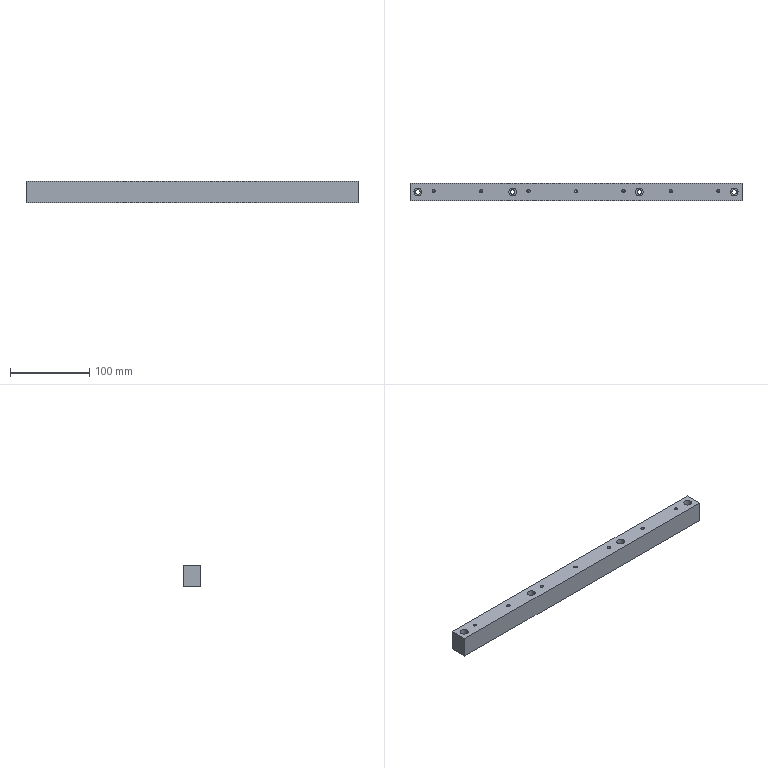Part | SolidWorks | features HoleWzd 2, Extrusion 1 | 1 solid | 54 faces | box 420 x 22 x 27 mm | volume 241946 mm3 | cylinder 30 | cone 14 | plane 10 | commonest cylinder face diameters 4.2 x14 5.5 x8 10 x8
STEP:
#1=CARTESIAN_POINT('',(-205.,0.,10.));
#2=VERTEX_POINT('',#1);
#3=CARTESIAN_POINT('',(-195.,0.,10.));
#4=VERTEX_POINT('',#3);
#5=CARTESIAN_POINT('',(-200.,0.,10.));
#6=DIRECTION('',(0.,0.,1.));
#7=DIRECTION('',(1.,0.,0.));
#8=AXIS2_PLACEMENT_3D('',#5,#6,#7);
#9=CIRCLE('',#8,5.);
#10=EDGE_CURVE('',#2,#4,#9,.T.);
#11=ORIENTED_EDGE('',*,*,#10,.F.);
#12=CARTESIAN_POINT('',(-205.,0.,27.));
#13=VERTEX_POINT('',#12);
#14=CARTESIAN_POINT('',(-205.,0.,27.));
#15=DIRECTION('',(0.,0.,1.));
#16=VECTOR('',#15,1000.);
#17=LINE('',#14,#16);
#18=EDGE_CURVE('',#2,#13,#17,.T.);
#19=ORIENTED_EDGE('',*,*,#18,.T.);
#20=CARTESIAN_POINT('',(-195.,0.,27.));
#21=VERTEX_POINT('',#20);
#22=CARTESIAN_POINT('',(-200.,0.,27.));
#23=DIRECTION('',(0.,0.,1.));
#24=DIRECTION('',(1.,0.,0.));
#25=AXIS2_PLACEMENT_3D('',#22,#23,#24);
#26=CIRCLE('',#25,5.);
#27=EDGE_CURVE('',#13,#21,#26,.T.);
#28=ORIENTED_EDGE('',*,*,#27,.T.);
#29=CARTESIAN_POINT('',(-195.,0.,27.));
#30=DIRECTION('',(0.,0.,1.));
#31=VECTOR('',#30,1000.);
#32=LINE('',#29,#31);
#33=EDGE_CURVE('',#4,#21,#32,.T.);
#34=ORIENTED_EDGE('',*,*,#33,.F.);
#35=EDGE_LOOP('',(#11,#19,#28,#34));
#36=FACE_OUTER_BOUND('',#35,.T.);
#37=CARTESIAN_POINT('',(-200.,0.,27.));
#38=DIRECTION('',(0.,0.,1.));
#39=DIRECTION('',(1.,0.,0.));
#40=AXIS2_PLACEMENT_3D('',#37,#38,#39);
#41=CYLINDRICAL_SURFACE('',#40,5.);
#42=ADVANCED_FACE('',(#36),#41,.F.);
#43=CARTESIAN_POINT('',(-202.75,0.,0.));
#44=VERTEX_POINT('',#43);
#45=CARTESIAN_POINT('',(-197.25,0.,0.));
#46=VERTEX_POINT('',#45);
#47=CARTESIAN_POINT('',(-200.,0.,0.));
#48=DIRECTION('',(0.,0.,1.));
#49=DIRECTION('',(1.,0.,0.));
#50=AXIS2_PLACEMENT_3D('',#47,#48,#49);
#51=CIRCLE('',#50,2.75);
#52=EDGE_CURVE('',#44,#46,#51,.T.);
#53=ORIENTED_EDGE('',*,*,#52,.F.);
#54=CARTESIAN_POINT('',(-202.75,0.,10.));
#55=VERTEX_POINT('',#54);
#56=CARTESIAN_POINT('',(-202.75,0.,27.));
#57=DIRECTION('',(0.,0.,1.));
#58=VECTOR('',#57,1000.);
#59=LINE('',#56,#58);
#60=EDGE_CURVE('',#44,#55,#59,.T.);
#61=ORIENTED_EDGE('',*,*,#60,.T.);
#62=CARTESIAN_POINT('',(-197.25,0.,10.));
#63=VERTEX_POINT('',#62);
#64=CARTESIAN_POINT('',(-200.,0.,10.));
#65=DIRECTION('',(0.,0.,1.));
#66=DIRECTION('',(1.,0.,0.));
#67=AXIS2_PLACEMENT_3D('',#64,#65,#66);
#68=CIRCLE('',#67,2.75);
#69=EDGE_CURVE('',#55,#63,#68,.T.);
#70=ORIENTED_EDGE('',*,*,#69,.T.);
#71=CARTESIAN_POINT('',(-197.25,0.,27.));
#72=DIRECTION('',(0.,0.,1.));
#73=VECTOR('',#72,1000.);
#74=LINE('',#71,#73);
#75=EDGE_CURVE('',#46,#63,#74,.T.);
#76=ORIENTED_EDGE('',*,*,#75,.F.);
#77=EDGE_LOOP('',(#53,#61,#70,#76));
#78=FACE_OUTER_BOUND('',#77,.T.);
#79=CARTESIAN_POINT('',(-200.,0.,27.));
#80=DIRECTION('',(0.,0.,1.));
#81=DIRECTION('',(1.,0.,0.));
#82=AXIS2_PLACEMENT_3D('',#79,#80,#81);
#83=CYLINDRICAL_SURFACE('',#82,2.75);
#84=ADVANCED_FACE('',(#78),#83,.F.);
#85=CARTESIAN_POINT('',(-85.,0.,10.));
#86=VERTEX_POINT('',#85);
#87=CARTESIAN_POINT('',(-75.,0.,10.));
#88=VERTEX_POINT('',#87);
#89=CARTESIAN_POINT('',(-80.,0.,10.));
#90=DIRECTION('',(0.,0.,1.));
#91=DIRECTION('',(1.,0.,0.));
#92=AXIS2_PLACEMENT_3D('',#89,#90,#91);
#93=CIRCLE('',#92,5.);
#94=EDGE_CURVE('',#86,#88,#93,.T.);
#95=ORIENTED_EDGE('',*,*,#94,.F.);
#96=CARTESIAN_POINT('',(-85.,0.,27.));
#97=VERTEX_POINT('',#96);
#98=CARTESIAN_POINT('',(-85.,0.,27.));
#99=DIRECTION('',(0.,0.,1.));
#100=VECTOR('',#99,1000.);
#101=LINE('',#98,#100);
#102=EDGE_CURVE('',#86,#97,#101,.T.);
#103=ORIENTED_EDGE('',*,*,#102,.T.);
#104=CARTESIAN_POINT('',(-75.,0.,27.));
#105=VERTEX_POINT('',#104);
#106=CARTESIAN_POINT('',(-80.,0.,27.));
#107=DIRECTION('',(0.,0.,1.));
#108=DIRECTION('',(1.,0.,0.));
#109=AXIS2_PLACEMENT_3D('',#106,#107,#108);
#110=CIRCLE('',#109,5.);
#111=EDGE_CURVE('',#97,#105,#110,.T.);
#112=ORIENTED_EDGE('',*,*,#111,.T.);
#113=CARTESIAN_POINT('',(-75.,0.,27.));
#114=DIRECTION('',(0.,0.,1.));
#115=VECTOR('',#114,1000.);
#116=LINE('',#113,#115);
#117=EDGE_CURVE('',#88,#105,#116,.T.);
#118=ORIENTED_EDGE('',*,*,#117,.F.);
#119=EDGE_LOOP('',(#95,#103,#112,#118));
#120=FACE_OUTER_BOUND('',#119,.T.);
#121=CARTESIAN_POINT('',(-80.,0.,27.));
#122=DIRECTION('',(0.,0.,1.));
#123=DIRECTION('',(1.,0.,0.));
#124=AXIS2_PLACEMENT_3D('',#121,#122,#123);
#125=CYLINDRICAL_SURFACE('',#124,5.);
#126=ADVANCED_FACE('',(#120),#125,.F.);
#127=CARTESIAN_POINT('',(-82.75,0.,0.));
#128=VERTEX_POINT('',#127);
#129=CARTESIAN_POINT('',(-77.25,0.,0.));
#130=VERTEX_POINT('',#129);
#131=CARTESIAN_POINT('',(-80.,0.,0.));
#132=DIRECTION('',(0.,0.,1.));
#133=DIRECTION('',(1.,0.,0.));
#134=AXIS2_PLACEMENT_3D('',#131,#132,#133);
#135=CIRCLE('',#134,2.75);
#136=EDGE_CURVE('',#128,#130,#135,.T.);
#137=ORIENTED_EDGE('',*,*,#136,.F.);
#138=CARTESIAN_POINT('',(-82.75,0.,10.));
#139=VERTEX_POINT('',#138);
#140=CARTESIAN_POINT('',(-82.75,0.,27.));
#141=DIRECTION('',(0.,0.,1.));
#142=VECTOR('',#141,1000.);
#143=LINE('',#140,#142);
#144=EDGE_CURVE('',#128,#139,#143,.T.);
#145=ORIENTED_EDGE('',*,*,#144,.T.);
#146=CARTESIAN_POINT('',(-77.25,0.,10.));
#147=VERTEX_POINT('',#146);
#148=CARTESIAN_POINT('',(-80.,0.,10.));
#149=DIRECTION('',(0.,0.,1.));
#150=DIRECTION('',(1.,0.,0.));
#151=AXIS2_PLACEMENT_3D('',#148,#149,#150);
#152=CIRCLE('',#151,2.75);
#153=EDGE_CURVE('',#139,#147,#152,.T.);
#154=ORIENTED_EDGE('',*,*,#153,.T.);
#155=CARTESIAN_POINT('',(-77.25,0.,27.));
#156=DIRECTION('',(0.,0.,1.));
#157=VECTOR('',#156,1000.);
#158=LINE('',#155,#157);
#159=EDGE_CURVE('',#130,#147,#158,.T.);
#160=ORIENTED_EDGE('',*,*,#159,.F.);
#161=EDGE_LOOP('',(#137,#145,#154,#160));
#162=FACE_OUTER_BOUND('',#161,.T.);
#163=CARTESIAN_POINT('',(-80.,0.,27.));
#164=DIRECTION('',(0.,0.,1.));
#165=DIRECTION('',(1.,0.,0.));
#166=AXIS2_PLACEMENT_3D('',#163,#164,#165);
#167=CYLINDRICAL_SURFACE('',#166,2.75);
#168=ADVANCED_FACE('',(#162),#167,.F.);
#169=CARTESIAN_POINT('',(75.,0.,10.));
#170=VERTEX_POINT('',#169);
#171=CARTESIAN_POINT('',(85.,0.,10.));
#172=VERTEX_POINT('',#171);
#173=CARTESIAN_POINT('',(80.,0.,10.));
#174=DIRECTION('',(0.,0.,1.));
#175=DIRECTION('',(1.,0.,0.));
#176=AXIS2_PLACEMENT_3D('',#173,#174,#175);
#177=CIRCLE('',#176,5.);
#178=EDGE_CURVE('',#170,#172,#177,.T.);
#179=ORIENTED_EDGE('',*,*,#178,.F.);
#180=CARTESIAN_POINT('',(75.,0.,27.));
#181=VERTEX_POINT('',#180);
#182=CARTESIAN_POINT('',(75.,0.,27.));
#183=DIRECTION('',(0.,0.,1.));
#184=VECTOR('',#183,1000.);
#185=LINE('',#182,#184);
#186=EDGE_CURVE('',#170,#181,#185,.T.);
#187=ORIENTED_EDGE('',*,*,#186,.T.);
#188=CARTESIAN_POINT('',(85.,0.,27.));
#189=VERTEX_POINT('',#188);
#190=CARTESIAN_POINT('',(80.,0.,27.));
#191=DIRECTION('',(0.,0.,1.));
#192=DIRECTION('',(1.,0.,0.));
#193=AXIS2_PLACEMENT_3D('',#190,#191,#192);
#194=CIRCLE('',#193,5.);
#195=EDGE_CURVE('',#181,#189,#194,.T.);
#196=ORIENTED_EDGE('',*,*,#195,.T.);
#197=CARTESIAN_POINT('',(85.,0.,27.));
#198=DIRECTION('',(0.,0.,1.));
#199=VECTOR('',#198,1000.);
#200=LINE('',#197,#199);
#201=EDGE_CURVE('',#172,#189,#200,.T.);
#202=ORIENTED_EDGE('',*,*,#201,.F.);
#203=EDGE_LOOP('',(#179,#187,#196,#202));
#204=FACE_OUTER_BOUND('',#203,.T.);
#205=CARTESIAN_POINT('',(80.,0.,27.));
#206=DIRECTION('',(0.,0.,1.));
#207=DIRECTION('',(1.,0.,0.));
#208=AXIS2_PLACEMENT_3D('',#205,#206,#207);
#209=CYLINDRICAL_SURFACE('',#208,5.);
#210=ADVANCED_FACE('',(#204),#209,.F.);
#211=CARTESIAN_POINT('',(77.25,0.,0.));
#212=VERTEX_POINT('',#211);
#213=CARTESIAN_POINT('',(82.75,0.,0.));
#214=VERTEX_POINT('',#213);
#215=CARTESIAN_POINT('',(80.,0.,0.));
#216=DIRECTION('',(0.,0.,1.));
#217=DIRECTION('',(1.,0.,0.));
#218=AXIS2_PLACEMENT_3D('',#215,#216,#217);
#219=CIRCLE('',#218,2.75);
#220=EDGE_CURVE('',#212,#214,#219,.T.);
#221=ORIENTED_EDGE('',*,*,#220,.F.);
#222=CARTESIAN_POINT('',(77.25,0.,10.));
#223=VERTEX_POINT('',#222);
#224=CARTESIAN_POINT('',(77.25,0.,27.));
#225=DIRECTION('',(0.,0.,1.));
#226=VECTOR('',#225,1000.);
#227=LINE('',#224,#226);
#228=EDGE_CURVE('',#212,#223,#227,.T.);
#229=ORIENTED_EDGE('',*,*,#228,.T.);
#230=CARTESIAN_POINT('',(82.75,0.,10.));
#231=VERTEX_POINT('',#230);
#232=CARTESIAN_POINT('',(80.,0.,10.));
#233=DIRECTION('',(0.,0.,1.));
#234=DIRECTION('',(1.,0.,0.));
#235=AXIS2_PLACEMENT_3D('',#232,#233,#234);
#236=CIRCLE('',#235,2.75);
#237=EDGE_CURVE('',#223,#231,#236,.T.);
#238=ORIENTED_EDGE('',*,*,#237,.T.);
#239=CARTESIAN_POINT('',(82.75,0.,27.));
#240=DIRECTION('',(0.,0.,1.));
#241=VECTOR('',#240,1000.);
#242=LINE('',#239,#241);
#243=EDGE_CURVE('',#214,#231,#242,.T.);
#244=ORIENTED_EDGE('',*,*,#243,.F.);
#245=EDGE_LOOP('',(#221,#229,#238,#244));
#246=FACE_OUTER_BOUND('',#245,.T.);
#247=CARTESIAN_POINT('',(80.,0.,27.));
#248=DIRECTION('',(0.,0.,1.));
#249=DIRECTION('',(1.,0.,0.));
#250=AXIS2_PLACEMENT_3D('',#247,#248,#249);
#251=CYLINDRICAL_SURFACE('',#250,2.75);
#252=ADVANCED_FACE('',(#246),#251,.F.);
#253=CARTESIAN_POINT('',(195.,0.,10.));
#254=VERTEX_POINT('',#253);
#255=CARTESIAN_POINT('',(205.,0.,10.));
#256=VERTEX_POINT('',#255);
#257=CARTESIAN_POINT('',(200.,0.,10.));
#258=DIRECTION('',(0.,0.,1.));
#259=DIRECTION('',(1.,0.,0.));
#260=AXIS2_PLACEMENT_3D('',#257,#258,#259);
#261=CIRCLE('',#260,5.);
#262=EDGE_CURVE('',#254,#256,#261,.T.);
#263=ORIENTED_EDGE('',*,*,#262,.F.);
#264=CARTESIAN_POINT('',(195.,0.,27.));
#265=VERTEX_POINT('',#264);
#266=CARTESIAN_POINT('',(195.,0.,27.));
#267=DIRECTION('',(0.,0.,1.));
#268=VECTOR('',#267,1000.);
#269=LINE('',#266,#268);
#270=EDGE_CURVE('',#254,#265,#269,.T.);
#271=ORIENTED_EDGE('',*,*,#270,.T.);
#272=CARTESIAN_POINT('',(205.,0.,27.));
#273=VERTEX_POINT('',#272);
#274=CARTESIAN_POINT('',(200.,0.,27.));
#275=DIRECTION('',(0.,0.,1.));
#276=DIRECTION('',(1.,0.,0.));
#277=AXIS2_PLACEMENT_3D('',#274,#275,#276);
#278=CIRCLE('',#277,5.);
#279=EDGE_CURVE('',#265,#273,#278,.T.);
#280=ORIENTED_EDGE('',*,*,#279,.T.);
#281=CARTESIAN_POINT('',(205.,0.,27.));
#282=DIRECTION('',(0.,0.,1.));
#283=VECTOR('',#282,1000.);
#284=LINE('',#281,#283);
#285=EDGE_CURVE('',#256,#273,#284,.T.);
#286=ORIENTED_EDGE('',*,*,#285,.F.);
#287=EDGE_LOOP('',(#263,#271,#280,#286));
#288=FACE_OUTER_BOUND('',#287,.T.);
#289=CARTESIAN_POINT('',(200.,0.,27.));
#290=DIRECTION('',(0.,0.,1.));
#291=DIRECTION('',(1.,0.,0.));
#292=AXIS2_PLACEMENT_3D('',#289,#290,#291);
#293=CYLINDRICAL_SURFACE('',#292,5.);
#294=ADVANCED_FACE('',(#288),#293,.F.);
#295=CARTESIAN_POINT('',(197.25,0.,0.));
#296=VERTEX_POINT('',#295);
#297=CARTESIAN_POINT('',(202.75,0.,0.));
#298=VERTEX_POINT('',#297);
#299=CARTESIAN_POINT('',(200.,0.,0.));
#300=DIRECTION('',(0.,0.,1.));
#301=DIRECTION('',(1.,0.,0.));
#302=AXIS2_PLACEMENT_3D('',#299,#300,#301);
#303=CIRCLE('',#302,2.75);
#304=EDGE_CURVE('',#296,#298,#303,.T.);
#305=ORIENTED_EDGE('',*,*,#304,.F.);
#306=CARTESIAN_POINT('',(197.25,0.,10.));
#307=VERTEX_POINT('',#306);
#308=CARTESIAN_POINT('',(197.25,0.,27.));
#309=DIRECTION('',(0.,0.,1.));
#310=VECTOR('',#309,1000.);
#311=LINE('',#308,#310);
#312=EDGE_CURVE('',#296,#307,#311,.T.);
#313=ORIENTED_EDGE('',*,*,#312,.T.);
#314=CARTESIAN_POINT('',(202.75,0.,10.));
#315=VERTEX_POINT('',#314);
#316=CARTESIAN_POINT('',(200.,0.,10.));
#317=DIRECTION('',(0.,0.,1.));
#318=DIRECTION('',(1.,0.,0.));
#319=AXIS2_PLACEMENT_3D('',#316,#317,#318);
#320=CIRCLE('',#319,2.75);
#321=EDGE_CURVE('',#307,#315,#320,.T.);
#322=ORIENTED_EDGE('',*,*,#321,.T.);
#323=CARTESIAN_POINT('',(202.75,0.,27.));
#324=DIRECTION('',(0.,0.,1.));
#325=VECTOR('',#324,1000.);
#326=LINE('',#323,#325);
#327=EDGE_CURVE('',#298,#315,#326,.T.);
#328=ORIENTED_EDGE('',*,*,#327,.F.);
#329=EDGE_LOOP('',(#305,#313,#322,#328));
#330=FACE_OUTER_BOUND('',#329,.T.);
#331=CARTESIAN_POINT('',(200.,0.,27.));
#332=DIRECTION('',(0.,0.,1.));
#333=DIRECTION('',(1.,0.,0.));
#334=AXIS2_PLACEMENT_3D('',#331,#332,#333);
#335=CYLINDRICAL_SURFACE('',#334,2.75);
#336=ADVANCED_FACE('',(#330),#335,.F.);
#337=CARTESIAN_POINT('',(-182.1,1.,14.6));
#338=VERTEX_POINT('',#337);
#339=CARTESIAN_POINT('',(-177.9,1.,14.6));
#340=VERTEX_POINT('',#339);
#341=CARTESIAN_POINT('',(-180.,1.,14.6));
#342=DIRECTION('',(0.,0.,1.));
#343=DIRECTION('',(1.,0.,0.));
#344=AXIS2_PLACEMENT_3D('',#341,#342,#343);
#345=CIRCLE('',#344,2.1);
#346=EDGE_CURVE('',#338,#340,#345,.T.);
#347=ORIENTED_EDGE('',*,*,#346,.F.);
#348=CARTESIAN_POINT('',(-182.1,1.,27.));
#349=VERTEX_POINT('',#348);
#350=CARTESIAN_POINT('',(-182.1,1.,27.));
#351=DIRECTION('',(0.,0.,1.));
#352=VECTOR('',#351,1000.);
#353=LINE('',#350,#352);
#354=EDGE_CURVE('',#338,#349,#353,.T.);
#355=ORIENTED_EDGE('',*,*,#354,.T.);
#356=CARTESIAN_POINT('',(-177.9,1.,27.));
#357=VERTEX_POINT('',#356);
#358=CARTESIAN_POINT('',(-180.,1.,27.));
#359=DIRECTION('',(0.,0.,1.));
#360=DIRECTION('',(1.,0.,0.));
#361=AXIS2_PLACEMENT_3D('',#358,#359,#360);
#362=CIRCLE('',#361,2.1);
#363=EDGE_CURVE('',#349,#357,#362,.T.);
#364=ORIENTED_EDGE('',*,*,#363,.T.);
#365=CARTESIAN_POINT('',(-177.9,1.,27.));
#366=DIRECTION('',(0.,0.,1.));
#367=VECTOR('',#366,1000.);
#368=LINE('',#365,#367);
#369=EDGE_CURVE('',#340,#357,#368,.T.);
#370=ORIENTED_EDGE('',*,*,#369,.F.);
#371=EDGE_LOOP('',(#347,#355,#364,#370));
#372=FACE_OUTER_BOUND('',#371,.T.);
#373=CARTESIAN_POINT('',(-180.,1.,27.));
#374=DIRECTION('',(0.,0.,1.));
#375=DIRECTION('',(1.,0.,0.));
#376=AXIS2_PLACEMENT_3D('',#373,#374,#375);
#377=CYLINDRICAL_SURFACE('',#376,2.1);
#378=ADVANCED_FACE('',(#372),#377,.F.);
#379=CARTESIAN_POINT('',(-180.,1.,13.338));
#380=VERTEX_POINT('',#379);
#381=CARTESIAN_POINT('',(-177.9,1.,14.6));
#382=DIRECTION('',(0.8572,0.,0.515));
#383=VECTOR('',#382,1000.);
#384=LINE('',#381,#383);
#385=EDGE_CURVE('',#380,#340,#384,.T.);
#386=ORIENTED_EDGE('',*,*,#385,.F.);
#387=CARTESIAN_POINT('',(-182.1,1.,14.6));
#388=DIRECTION('',(-0.8572,0.,0.515));
#389=VECTOR('',#388,1000.);
#390=LINE('',#387,#389);
#391=EDGE_CURVE('',#380,#338,#390,.T.);
#392=ORIENTED_EDGE('',*,*,#391,.T.);
#393=ORIENTED_EDGE('',*,*,#346,.T.);
#394=EDGE_LOOP('',(#386,#392,#393));
#395=FACE_OUTER_BOUND('',#394,.T.);
#396=CARTESIAN_POINT('',(-180.,1.,14.6));
#397=DIRECTION('',(0.,0.,1.));
#398=DIRECTION('',(1.,0.,0.));
#399=AXIS2_PLACEMENT_3D('',#396,#397,#398);
#400=CONICAL_SURFACE('',#399,2.1,1.03);
#401=ADVANCED_FACE('',(#395),#400,.F.);
#402=CARTESIAN_POINT('',(-122.1,1.,14.6));
#403=VERTEX_POINT('',#402);
#404=CARTESIAN_POINT('',(-117.9,1.,14.6));
#405=VERTEX_POINT('',#404);
#406=CARTESIAN_POINT('',(-120.,1.,14.6));
#407=DIRECTION('',(0.,0.,1.));
#408=DIRECTION('',(1.,0.,0.));
#409=AXIS2_PLACEMENT_3D('',#406,#407,#408);
#410=CIRCLE('',#409,2.1);
#411=EDGE_CURVE('',#403,#405,#410,.T.);
#412=ORIENTED_EDGE('',*,*,#411,.F.);
#413=CARTESIAN_POINT('',(-122.1,1.,27.));
#414=VERTEX_POINT('',#413);
#415=CARTESIAN_POINT('',(-122.1,1.,27.));
#416=DIRECTION('',(0.,0.,1.));
#417=VECTOR('',#416,1000.);
#418=LINE('',#415,#417);
#419=EDGE_CURVE('',#403,#414,#418,.T.);
#420=ORIENTED_EDGE('',*,*,#419,.T.);
#421=CARTESIAN_POINT('',(-117.9,1.,27.));
#422=VERTEX_POINT('',#421);
#423=CARTESIAN_POINT('',(-120.,1.,27.));
#424=DIRECTION('',(0.,0.,1.));
#425=DIRECTION('',(1.,0.,0.));
#426=AXIS2_PLACEMENT_3D('',#423,#424,#425);
#427=CIRCLE('',#426,2.1);
#428=EDGE_CURVE('',#414,#422,#427,.T.);
#429=ORIENTED_EDGE('',*,*,#428,.T.);
#430=CARTESIAN_POINT('',(-117.9,1.,27.));
#431=DIRECTION('',(0.,0.,1.));
#432=VECTOR('',#431,1000.);
#433=LINE('',#430,#432);
#434=EDGE_CURVE('',#405,#422,#433,.T.);
#435=ORIENTED_EDGE('',*,*,#434,.F.);
#436=EDGE_LOOP('',(#412,#420,#429,#435));
#437=FACE_OUTER_BOUND('',#436,.T.);
#438=CARTESIAN_POINT('',(-120.,1.,27.));
#439=DIRECTION('',(0.,0.,1.));
#440=DIRECTION('',(1.,0.,0.));
#441=AXIS2_PLACEMENT_3D('',#438,#439,#440);
#442=CYLINDRICAL_SURFACE('',#441,2.1);
#443=ADVANCED_FACE('',(#437),#442,.F.);
#444=CARTESIAN_POINT('',(-120.,1.,13.338));
#445=VERTEX_POINT('',#444);
#446=CARTESIAN_POINT('',(-117.9,1.,14.6));
#447=DIRECTION('',(0.8572,0.,0.515));
#448=VECTOR('',#447,1000.);
#449=LINE('',#446,#448);
#450=EDGE_CURVE('',#445,#405,#449,.T.);
#451=ORIENTED_EDGE('',*,*,#450,.F.);
#452=CARTESIAN_POINT('',(-122.1,1.,14.6));
#453=DIRECTION('',(-0.8572,0.,0.515));
#454=VECTOR('',#453,1000.);
#455=LINE('',#452,#454);
#456=EDGE_CURVE('',#445,#403,#455,.T.);
#457=ORIENTED_EDGE('',*,*,#456,.T.);
#458=ORIENTED_EDGE('',*,*,#411,.T.);
#459=EDGE_LOOP('',(#451,#457,#458));
#460=FACE_OUTER_BOUND('',#459,.T.);
#461=CARTESIAN_POINT('',(-120.,1.,14.6));
#462=DIRECTION('',(0.,0.,1.));
#463=DIRECTION('',(1.,0.,0.));
#464=AXIS2_PLACEMENT_3D('',#461,#462,#463);
#465=CONICAL_SURFACE('',#464,2.1,1.03);
#466=ADVANCED_FACE('',(#460),#465,.F.);
#467=CARTESIAN_POINT('',(-62.1,1.,14.6));
#468=VERTEX_POINT('',#467);
#469=CARTESIAN_POINT('',(-57.9,1.,14.6));
#470=VERTEX_POINT('',#469);
#471=CARTESIAN_POINT('',(-60.,1.,14.6));
#472=DIRECTION('',(0.,0.,1.));
#473=DIRECTION('',(1.,0.,0.));
#474=AXIS2_PLACEMENT_3D('',#471,#472,#473);
#475=CIRCLE('',#474,2.1);
#476=EDGE_CURVE('',#468,#470,#475,.T.);
#477=ORIENTED_EDGE('',*,*,#476,.F.);
#478=CARTESIAN_POINT('',(-62.1,1.,27.));
#479=VERTEX_POINT('',#478);
#480=CARTESIAN_POINT('',(-62.1,1.,27.));
#481=DIRECTION('',(0.,0.,1.));
#482=VECTOR('',#481,1000.);
#483=LINE('',#480,#482);
#484=EDGE_CURVE('',#468,#479,#483,.T.);
#485=ORIENTED_EDGE('',*,*,#484,.T.);
#486=CARTESIAN_POINT('',(-57.9,1.,27.));
#487=VERTEX_POINT('',#486);
#488=CARTESIAN_POINT('',(-60.,1.,27.));
#489=DIRECTION('',(0.,0.,1.));
#490=DIRECTION('',(1.,0.,0.));
#491=AXIS2_PLACEMENT_3D('',#488,#489,#490);
#492=CIRCLE('',#491,2.1);
#493=EDGE_CURVE('',#479,#487,#492,.T.);
#494=ORIENTED_EDGE('',*,*,#493,.T.);
#495=CARTESIAN_POINT('',(-57.9,1.,27.));
#496=DIRECTION('',(0.,0.,1.));
#497=VECTOR('',#496,1000.);
#498=LINE('',#495,#497);
#499=EDGE_CURVE('',#470,#487,#498,.T.);
#500=ORIENTED_EDGE('',*,*,#499,.F.);
#501=EDGE_LOOP('',(#477,#485,#494,#500));
#502=FACE_OUTER_BOUND('',#501,.T.);
#503=CARTESIAN_POINT('',(-60.,1.,27.));
#504=DIRECTION('',(0.,0.,1.));
#505=DIRECTION('',(1.,0.,0.));
#506=AXIS2_PLACEMENT_3D('',#503,#504,#505);
#507=CYLINDRICAL_SURFACE('',#506,2.1);
#508=ADVANCED_FACE('',(#502),#507,.F.);
#509=CARTESIAN_POINT('',(-60.,1.,13.338));
#510=VERTEX_POINT('',#509);
#511=CARTESIAN_POINT('',(-57.9,1.,14.6));
#512=DIRECTION('',(0.8572,0.,0.515));
#513=VECTOR('',#512,1000.);
#514=LINE('',#511,#513);
#515=EDGE_CURVE('',#510,#470,#514,.T.);
#516=ORIENTED_EDGE('',*,*,#515,.F.);
#517=CARTESIAN_POINT('',(-62.1,1.,14.6));
#518=DIRECTION('',(-0.8572,0.,0.515));
#519=VECTOR('',#518,1000.);
#520=LINE('',#517,#519);
#521=EDGE_CURVE('',#510,#468,#520,.T.);
#522=ORIENTED_EDGE('',*,*,#521,.T.);
#523=ORIENTED_EDGE('',*,*,#476,.T.);
#524=EDGE_LOOP('',(#516,#522,#523));
#525=FACE_OUTER_BOUND('',#524,.T.);
#526=CARTESIAN_POINT('',(-60.,1.,14.6));
#527=DIRECTION('',(0.,0.,1.));
#528=DIRECTION('',(1.,0.,0.));
#529=AXIS2_PLACEMENT_3D('',#526,#527,#528);
#530=CONICAL_SURFACE('',#529,2.1,1.03);
#531=ADVANCED_FACE('',(#525),#530,.F.);
#532=CARTESIAN_POINT('',(-2.1,1.,14.6));
#533=VERTEX_POINT('',#532);
#534=CARTESIAN_POINT('',(2.1,1.,14.6));
#535=VERTEX_POINT('',#534);
#536=CARTESIAN_POINT('',(0.,1.,14.6));
#537=DIRECTION('',(0.,0.,1.));
#538=DIRECTION('',(1.,0.,0.));
#539=AXIS2_PLACEMENT_3D('',#536,#537,#538);
#540=CIRCLE('',#539,2.1);
#541=EDGE_CURVE('',#533,#535,#540,.T.);
#542=ORIENTED_EDGE('',*,*,#541,.F.);
#543=CARTESIAN_POINT('',(-2.1,1.,27.));
#544=VERTEX_POINT('',#543);
#545=CARTESIAN_POINT('',(-2.1,1.,27.));
#546=DIRECTION('',(0.,0.,1.));
#547=VECTOR('',#546,1000.);
#548=LINE('',#545,#547);
#549=EDGE_CURVE('',#533,#544,#548,.T.);
#550=ORIENTED_EDGE('',*,*,#549,.T.);
#551=CARTESIAN_POINT('',(2.1,1.,27.));
#552=VERTEX_POINT('',#551);
#553=CARTESIAN_POINT('',(0.,1.,27.));
#554=DIRECTION('',(0.,0.,1.));
#555=DIRECTION('',(1.,0.,0.));
#556=AXIS2_PLACEMENT_3D('',#553,#554,#555);
#557=CIRCLE('',#556,2.1);
#558=EDGE_CURVE('',#544,#552,#557,.T.);
#559=ORIENTED_EDGE('',*,*,#558,.T.);
#560=CARTESIAN_POINT('',(2.1,1.,27.));
#561=DIRECTION('',(0.,0.,1.));
#562=VECTOR('',#561,1000.);
#563=LINE('',#560,#562);
#564=EDGE_CURVE('',#535,#552,#563,.T.);
#565=ORIENTED_EDGE('',*,*,#564,.F.);
#566=EDGE_LOOP('',(#542,#550,#559,#565));
#567=FACE_OUTER_BOUND('',#566,.T.);
#568=CARTESIAN_POINT('',(0.,1.,27.));
#569=DIRECTION('',(0.,0.,1.));
#570=DIRECTION('',(1.,0.,0.));
#571=AXIS2_PLACEMENT_3D('',#568,#569,#570);
#572=CYLINDRICAL_SURFACE('',#571,2.1);
#573=ADVANCED_FACE('',(#567),#572,.F.);
#574=CARTESIAN_POINT('',(0.,1.,13.338));
#575=VERTEX_POINT('',#574);
#576=CARTESIAN_POINT('',(2.1,1.,14.6));
#577=DIRECTION('',(0.8572,0.,0.515));
#578=VECTOR('',#577,1000.);
#579=LINE('',#576,#578);
#580=EDGE_CURVE('',#575,#535,#579,.T.);
#581=ORIENTED_EDGE('',*,*,#580,.F.);
#582=CARTESIAN_POINT('',(-2.1,1.,14.6));
#583=DIRECTION('',(-0.8572,0.,0.515));
#584=VECTOR('',#583,1000.);
#585=LINE('',#582,#584);
#586=EDGE_CURVE('',#575,#533,#585,.T.);
#587=ORIENTED_EDGE('',*,*,#586,.T.);
#588=ORIENTED_EDGE('',*,*,#541,.T.);
#589=EDGE_LOOP('',(#581,#587,#588));
#590=FACE_OUTER_BOUND('',#589,.T.);
#591=CARTESIAN_POINT('',(0.,1.,14.6));
#592=DIRECTION('',(0.,0.,1.));
#593=DIRECTION('',(1.,0.,0.));
#594=AXIS2_PLACEMENT_3D('',#591,#592,#593);
#595=CONICAL_SURFACE('',#594,2.1,1.03);
#596=ADVANCED_FACE('',(#590),#595,.F.);
#597=CARTESIAN_POINT('',(57.9,1.,14.6));
#598=VERTEX_POINT('',#597);
#599=CARTESIAN_POINT('',(62.1,1.,14.6));
#600=VERTEX_POINT('',#599);
#601=CARTESIAN_POINT('',(60.,1.,14.6));
#602=DIRECTION('',(0.,0.,1.));
#603=DIRECTION('',(1.,0.,0.));
#604=AXIS2_PLACEMENT_3D('',#601,#602,#603);
#605=CIRCLE('',#604,2.1);
#606=EDGE_CURVE('',#598,#600,#605,.T.);
#607=ORIENTED_EDGE('',*,*,#606,.F.);
#608=CARTESIAN_POINT('',(57.9,1.,27.));
#609=VERTEX_POINT('',#608);
#610=CARTESIAN_POINT('',(57.9,1.,27.));
#611=DIRECTION('',(0.,0.,1.));
#612=VECTOR('',#611,1000.);
#613=LINE('',#610,#612);
#614=EDGE_CURVE('',#598,#609,#613,.T.);
#615=ORIENTED_EDGE('',*,*,#614,.T.);
#616=CARTESIAN_POINT('',(62.1,1.,27.));
#617=VERTEX_POINT('',#616);
#618=CARTESIAN_POINT('',(60.,1.,27.));
#619=DIRECTION('',(0.,0.,1.));
#620=DIRECTION('',(1.,0.,0.));
#621=AXIS2_PLACEMENT_3D('',#618,#619,#620);
#622=CIRCLE('',#621,2.1);
#623=EDGE_CURVE('',#609,#617,#622,.T.);
#624=ORIENTED_EDGE('',*,*,#623,.T.);
#625=CARTESIAN_POINT('',(62.1,1.,27.));
#626=DIRECTION('',(0.,0.,1.));
#627=VECTOR('',#626,1000.);
#628=LINE('',#625,#627);
#629=EDGE_CURVE('',#600,#617,#628,.T.);
#630=ORIENTED_EDGE('',*,*,#629,.F.);
#631=EDGE_LOOP('',(#607,#615,#624,#630));
#632=FACE_OUTER_BOUND('',#631,.T.);
#633=CARTESIAN_POINT('',(60.,1.,27.));
#634=DIRECTION('',(0.,0.,1.));
#635=DIRECTION('',(1.,0.,0.));
#636=AXIS2_PLACEMENT_3D('',#633,#634,#635);
#637=CYLINDRICAL_SURFACE('',#636,2.1);
#638=ADVANCED_FACE('',(#632),#637,.F.);
#639=CARTESIAN_POINT('',(60.,1.,13.338));
#640=VERTEX_POINT('',#639);
#641=CARTESIAN_POINT('',(62.1,1.,14.6));
#642=DIRECTION('',(0.8572,0.,0.515));
#643=VECTOR('',#642,1000.);
#644=LINE('',#641,#643);
#645=EDGE_CURVE('',#640,#600,#644,.T.);
#646=ORIENTED_EDGE('',*,*,#645,.F.);
#647=CARTESIAN_POINT('',(57.9,1.,14.6));
#648=DIRECTION('',(-0.8572,0.,0.515));
#649=VECTOR('',#648,1000.);
#650=LINE('',#647,#649);
#651=EDGE_CURVE('',#640,#598,#650,.T.);
#652=ORIENTED_EDGE('',*,*,#651,.T.);
#653=ORIENTED_EDGE('',*,*,#606,.T.);
#654=EDGE_LOOP('',(#646,#652,#653));
#655=FACE_OUTER_BOUND('',#654,.T.);
#656=CARTESIAN_POINT('',(60.,1.,14.6));
#657=DIRECTION('',(0.,0.,1.));
#658=DIRECTION('',(1.,0.,0.));
#659=AXIS2_PLACEMENT_3D('',#656,#657,#658);
#660=CONICAL_SURFACE('',#659,2.1,1.03);
#661=ADVANCED_FACE('',(#655),#660,.F.);
#662=CARTESIAN_POINT('',(117.9,1.,14.6));
#663=VERTEX_POINT('',#662);
#664=CARTESIAN_POINT('',(122.1,1.,14.6));
#665=VERTEX_POINT('',#664);
#666=CARTESIAN_POINT('',(120.,1.,14.6));
#667=DIRECTION('',(0.,0.,1.));
#668=DIRECTION('',(1.,0.,0.));
#669=AXIS2_PLACEMENT_3D('',#666,#667,#668);
#670=CIRCLE('',#669,2.1);
#671=EDGE_CURVE('',#663,#665,#670,.T.);
#672=ORIENTED_EDGE('',*,*,#671,.F.);
#673=CARTESIAN_POINT('',(117.9,1.,27.));
#674=VERTEX_POINT('',#673);
#675=CARTESIAN_POINT('',(117.9,1.,27.));
#676=DIRECTION('',(0.,0.,1.));
#677=VECTOR('',#676,1000.);
#678=LINE('',#675,#677);
#679=EDGE_CURVE('',#663,#674,#678,.T.);
#680=ORIENTED_EDGE('',*,*,#679,.T.);
#681=CARTESIAN_POINT('',(122.1,1.,27.));
#682=VERTEX_POINT('',#681);
#683=CARTESIAN_POINT('',(120.,1.,27.));
#684=DIRECTION('',(0.,0.,1.));
#685=DIRECTION('',(1.,0.,0.));
#686=AXIS2_PLACEMENT_3D('',#683,#684,#685);
#687=CIRCLE('',#686,2.1);
#688=EDGE_CURVE('',#674,#682,#687,.T.);
#689=ORIENTED_EDGE('',*,*,#688,.T.);
#690=CARTESIAN_POINT('',(122.1,1.,27.));
#691=DIRECTION('',(0.,0.,1.));
#692=VECTOR('',#691,1000.);
#693=LINE('',#690,#692);
#694=EDGE_CURVE('',#665,#682,#693,.T.);
#695=ORIENTED_EDGE('',*,*,#694,.F.);
#696=EDGE_LOOP('',(#672,#680,#689,#695));
#697=FACE_OUTER_BOUND('',#696,.T.);
#698=CARTESIAN_POINT('',(120.,1.,27.));
#699=DIRECTION('',(0.,0.,1.));
#700=DIRECTION('',(1.,0.,0.));
#701=AXIS2_PLACEMENT_3D('',#698,#699,#700);
#702=CYLINDRICAL_SURFACE('',#701,2.1);
#703=ADVANCED_FACE('',(#697),#702,.F.);
#704=CARTESIAN_POINT('',(120.,1.,13.338));
#705=VERTEX_POINT('',#704);
#706=CARTESIAN_POINT('',(122.1,1.,14.6));
#707=DIRECTION('',(0.8572,0.,0.515));
#708=VECTOR('',#707,1000.);
#709=LINE('',#706,#708);
#710=EDGE_CURVE('',#705,#665,#709,.T.);
#711=ORIENTED_EDGE('',*,*,#710,.F.);
#712=CARTESIAN_POINT('',(117.9,1.,14.6));
#713=DIRECTION('',(-0.8572,0.,0.515));
#714=VECTOR('',#713,1000.);
#715=LINE('',#712,#714);
#716=EDGE_CURVE('',#705,#663,#715,.T.);
#717=ORIENTED_EDGE('',*,*,#716,.T.);
#718=ORIENTED_EDGE('',*,*,#671,.T.);
#719=EDGE_LOOP('',(#711,#717,#718));
#720=FACE_OUTER_BOUND('',#719,.T.);
#721=CARTESIAN_POINT('',(120.,1.,14.6));
#722=DIRECTION('',(0.,0.,1.));
#723=DIRECTION('',(1.,0.,0.));
#724=AXIS2_PLACEMENT_3D('',#721,#722,#723);
#725=CONICAL_SURFACE('',#724,2.1,1.03);
#726=ADVANCED_FACE('',(#720),#725,.F.);
#727=CARTESIAN_POINT('',(177.9,1.,14.6));
#728=VERTEX_POINT('',#727);
#729=CARTESIAN_POINT('',(182.1,1.,14.6));
#730=VERTEX_POINT('',#729);
#731=CARTESIAN_POINT('',(180.,1.,14.6));
#732=DIRECTION('',(0.,0.,1.));
#733=DIRECTION('',(1.,0.,0.));
#734=AXIS2_PLACEMENT_3D('',#731,#732,#733);
#735=CIRCLE('',#734,2.1);
#736=EDGE_CURVE('',#728,#730,#735,.T.);
#737=ORIENTED_EDGE('',*,*,#736,.F.);
#738=CARTESIAN_POINT('',(177.9,1.,27.));
#739=VERTEX_POINT('',#738);
#740=CARTESIAN_POINT('',(177.9,1.,27.));
#741=DIRECTION('',(0.,0.,1.));
#742=VECTOR('',#741,1000.);
#743=LINE('',#740,#742);
#744=EDGE_CURVE('',#728,#739,#743,.T.);
#745=ORIENTED_EDGE('',*,*,#744,.T.);
#746=CARTESIAN_POINT('',(182.1,1.,27.));
#747=VERTEX_POINT('',#746);
#748=CARTESIAN_POINT('',(180.,1.,27.));
#749=DIRECTION('',(0.,0.,1.));
#750=DIRECTION('',(1.,0.,0.));
#751=AXIS2_PLACEMENT_3D('',#748,#749,#750);
#752=CIRCLE('',#751,2.1);
#753=EDGE_CURVE('',#739,#747,#752,.T.);
#754=ORIENTED_EDGE('',*,*,#753,.T.);
#755=CARTESIAN_POINT('',(182.1,1.,27.));
#756=DIRECTION('',(0.,0.,1.));
#757=VECTOR('',#756,1000.);
#758=LINE('',#755,#757);
#759=EDGE_CURVE('',#730,#747,#758,.T.);
#760=ORIENTED_EDGE('',*,*,#759,.F.);
#761=EDGE_LOOP('',(#737,#745,#754,#760));
#762=FACE_OUTER_BOUND('',#761,.T.);
#763=CARTESIAN_POINT('',(180.,1.,27.));
#764=DIRECTION('',(0.,0.,1.));
#765=DIRECTION('',(1.,0.,0.));
#766=AXIS2_PLACEMENT_3D('',#763,#764,#765);
#767=CYLINDRICAL_SURFACE('',#766,2.1);
#768=ADVANCED_FACE('',(#762),#767,.F.);
#769=CARTESIAN_POINT('',(180.,1.,13.338));
#770=VERTEX_POINT('',#769);
#771=CARTESIAN_POINT('',(182.1,1.,14.6));
#772=DIRECTION('',(0.8572,0.,0.515));
#773=VECTOR('',#772,1000.);
#774=LINE('',#771,#773);
#775=EDGE_CURVE('',#770,#730,#774,.T.);
#776=ORIENTED_EDGE('',*,*,#775,.F.);
#777=CARTESIAN_POINT('',(177.9,1.,14.6));
#778=DIRECTION('',(-0.8572,0.,0.515));
#779=VECTOR('',#778,1000.);
#780=LINE('',#777,#779);
#781=EDGE_CURVE('',#770,#728,#780,.T.);
#782=ORIENTED_EDGE('',*,*,#781,.T.);
#783=ORIENTED_EDGE('',*,*,#736,.T.);
#784=EDGE_LOOP('',(#776,#782,#783));
#785=FACE_OUTER_BOUND('',#784,.T.);
#786=CARTESIAN_POINT('',(180.,1.,14.6));
#787=DIRECTION('',(0.,0.,1.));
#788=DIRECTION('',(1.,0.,0.));
#789=AXIS2_PLACEMENT_3D('',#786,#787,#788);
#790=CONICAL_SURFACE('',#789,2.1,1.03);
#791=ADVANCED_FACE('',(#785),#790,.F.);
#792=CARTESIAN_POINT('',(210.,-11.,0.));
#793=VERTEX_POINT('',#792);
#794=CARTESIAN_POINT('',(210.,11.,0.));
#795=VERTEX_POINT('',#794);
#796=CARTESIAN_POINT('',(210.,-11.,0.));
#797=DIRECTION('',(0.,1.,0.));
#798=VECTOR('',#797,1000.);
#799=LINE('',#796,#798);
#800=EDGE_CURVE('',#793,#795,#799,.T.);
#801=ORIENTED_EDGE('',*,*,#800,.T.);
#802=CARTESIAN_POINT('',(210.,11.,27.));
#803=VERTEX_POINT('',#802);
#804=CARTESIAN_POINT('',(210.,11.,27.));
#805=DIRECTION('',(0.,0.,-1.));
#806=VECTOR('',#805,1000.);
#807=LINE('',#804,#806);
#808=EDGE_CURVE('',#803,#795,#807,.T.);
#809=ORIENTED_EDGE('',*,*,#808,.F.);
#810=CARTESIAN_POINT('',(210.,-11.,27.));
#811=VERTEX_POINT('',#810);
#812=CARTESIAN_POINT('',(210.,-11.,27.));
#813=DIRECTION('',(0.,1.,0.));
#814=VECTOR('',#813,1000.);
#815=LINE('',#812,#814);
#816=EDGE_CURVE('',#811,#803,#815,.T.);
#817=ORIENTED_EDGE('',*,*,#816,.F.);
#818=CARTESIAN_POINT('',(210.,-11.,27.));
#819=DIRECTION('',(0.,0.,-1.));
#820=VECTOR('',#819,1000.);
#821=LINE('',#818,#820);
#822=EDGE_CURVE('',#811,#793,#821,.T.);
#823=ORIENTED_EDGE('',*,*,#822,.T.);
#824=EDGE_LOOP('',(#801,#809,#817,#823));
#825=FACE_OUTER_BOUND('',#824,.T.);
#826=CARTESIAN_POINT('',(210.,-11.,27.));
#827=DIRECTION('',(-1.,0.,0.));
#828=DIRECTION('',(0.,0.,1.));
#829=AXIS2_PLACEMENT_3D('',#826,#827,#828);
#830=PLANE('',#829);
#831=ADVANCED_FACE('',(#825),#830,.F.);
#832=CARTESIAN_POINT('',(-210.,11.,0.));
#833=VERTEX_POINT('',#832);
#834=CARTESIAN_POINT('',(-210.,11.,0.));
#835=DIRECTION('',(-1.,0.,0.));
#836=VECTOR('',#835,1000.);
#837=LINE('',#834,#836);
#838=EDGE_CURVE('',#795,#833,#837,.T.);
#839=ORIENTED_EDGE('',*,*,#838,.T.);
#840=CARTESIAN_POINT('',(-210.,11.,27.));
#841=VERTEX_POINT('',#840);
#842=CARTESIAN_POINT('',(-210.,11.,27.));
#843=DIRECTION('',(0.,0.,-1.));
#844=VECTOR('',#843,1000.);
#845=LINE('',#842,#844);
#846=EDGE_CURVE('',#841,#833,#845,.T.);
#847=ORIENTED_EDGE('',*,*,#846,.F.);
#848=CARTESIAN_POINT('',(-210.,11.,27.));
#849=DIRECTION('',(-1.,0.,0.));
#850=VECTOR('',#849,1000.);
#851=LINE('',#848,#850);
#852=EDGE_CURVE('',#803,#841,#851,.T.);
#853=ORIENTED_EDGE('',*,*,#852,.F.);
#854=ORIENTED_EDGE('',*,*,#808,.T.);
#855=EDGE_LOOP('',(#839,#847,#853,#854));
#856=FACE_OUTER_BOUND('',#855,.T.);
#857=CARTESIAN_POINT('',(-210.,11.,27.));
#858=DIRECTION('',(0.,-1.,0.));
#859=DIRECTION('',(0.,0.,-1.));
#860=AXIS2_PLACEMENT_3D('',#857,#858,#859);
#861=PLANE('',#860);
#862=ADVANCED_FACE('',(#856),#861,.F.);
#863=CARTESIAN_POINT('',(-210.,-11.,0.));
#864=VERTEX_POINT('',#863);
#865=CARTESIAN_POINT('',(-210.,-11.,0.));
#866=DIRECTION('',(0.,-1.,0.));
#867=VECTOR('',#866,1000.);
#868=LINE('',#865,#867);
#869=EDGE_CURVE('',#833,#864,#868,.T.);
#870=ORIENTED_EDGE('',*,*,#869,.T.);
#871=CARTESIAN_POINT('',(-210.,-11.,27.));
#872=VERTEX_POINT('',#871);
#873=CARTESIAN_POINT('',(-210.,-11.,27.));
#874=DIRECTION('',(0.,0.,-1.));
#875=VECTOR('',#874,1000.);
#876=LINE('',#873,#875);
#877=EDGE_CURVE('',#872,#864,#876,.T.);
#878=ORIENTED_EDGE('',*,*,#877,.F.);
#879=CARTESIAN_POINT('',(-210.,-11.,27.));
#880=DIRECTION('',(0.,-1.,0.));
#881=VECTOR('',#880,1000.);
#882=LINE('',#879,#881);
#883=EDGE_CURVE('',#841,#872,#882,.T.);
#884=ORIENTED_EDGE('',*,*,#883,.F.);
#885=ORIENTED_EDGE('',*,*,#846,.T.);
#886=EDGE_LOOP('',(#870,#878,#884,#885));
#887=FACE_OUTER_BOUND('',#886,.T.);
#888=CARTESIAN_POINT('',(-210.,-11.,27.));
#889=DIRECTION('',(1.,0.,0.));
#890=DIRECTION('',(0.,0.,-1.));
#891=AXIS2_PLACEMENT_3D('',#888,#889,#890);
#892=PLANE('',#891);
#893=ADVANCED_FACE('',(#887),#892,.F.);
#894=CARTESIAN_POINT('',(-210.,-11.,0.));
#895=DIRECTION('',(1.,0.,0.));
#896=VECTOR('',#895,1000.);
#897=LINE('',#894,#896);
#898=EDGE_CURVE('',#864,#793,#897,.T.);
#899=ORIENTED_EDGE('',*,*,#898,.T.);
#900=ORIENTED_EDGE('',*,*,#822,.F.);
#901=CARTESIAN_POINT('',(-210.,-11.,27.));
#902=DIRECTION('',(1.,0.,0.));
#903=VECTOR('',#902,1000.);
#904=LINE('',#901,#903);
#905=EDGE_CURVE('',#872,#811,#904,.T.);
#906=ORIENTED_EDGE('',*,*,#905,.F.);
#907=ORIENTED_EDGE('',*,*,#877,.T.);
#908=EDGE_LOOP('',(#899,#900,#906,#907));
#909=FACE_OUTER_BOUND('',#908,.T.);
#910=CARTESIAN_POINT('',(-210.,-11.,27.));
#911=DIRECTION('',(0.,1.,0.));
#912=DIRECTION('',(0.,0.,1.));
#913=AXIS2_PLACEMENT_3D('',#910,#911,#912);
#914=PLANE('',#913);
#915=ADVANCED_FACE('',(#909),#914,.F.);
#916=CARTESIAN_POINT('',(-200.,0.,27.));
#917=DIRECTION('',(0.,0.,1.));
#918=DIRECTION('',(1.,0.,0.));
#919=AXIS2_PLACEMENT_3D('',#916,#917,#918);
#920=CIRCLE('',#919,5.);
#921=EDGE_CURVE('',#21,#13,#920,.T.);
#922=ORIENTED_EDGE('',*,*,#921,.F.);
#923=ORIENTED_EDGE('',*,*,#27,.F.);
#924=EDGE_LOOP('',(#922,#923));
#925=FACE_BOUND('',#924,.T.);
#926=CARTESIAN_POINT('',(-80.,0.,27.));
#927=DIRECTION('',(0.,0.,1.));
#928=DIRECTION('',(1.,0.,0.));
#929=AXIS2_PLACEMENT_3D('',#926,#927,#928);
#930=CIRCLE('',#929,5.);
#931=EDGE_CURVE('',#105,#97,#930,.T.);
#932=ORIENTED_EDGE('',*,*,#931,.F.);
#933=ORIENTED_EDGE('',*,*,#111,.F.);
#934=EDGE_LOOP('',(#932,#933));
#935=FACE_BOUND('',#934,.T.);
#936=CARTESIAN_POINT('',(80.,0.,27.));
#937=DIRECTION('',(0.,0.,1.));
#938=DIRECTION('',(1.,0.,0.));
#939=AXIS2_PLACEMENT_3D('',#936,#937,#938);
#940=CIRCLE('',#939,5.);
#941=EDGE_CURVE('',#189,#181,#940,.T.);
#942=ORIENTED_EDGE('',*,*,#941,.F.);
#943=ORIENTED_EDGE('',*,*,#195,.F.);
#944=EDGE_LOOP('',(#942,#943));
#945=FACE_BOUND('',#944,.T.);
#946=CARTESIAN_POINT('',(200.,0.,27.));
#947=DIRECTION('',(0.,0.,1.));
#948=DIRECTION('',(1.,0.,0.));
#949=AXIS2_PLACEMENT_3D('',#946,#947,#948);
#950=CIRCLE('',#949,5.);
#951=EDGE_CURVE('',#273,#265,#950,.T.);
#952=ORIENTED_EDGE('',*,*,#951,.F.);
#953=ORIENTED_EDGE('',*,*,#279,.F.);
#954=EDGE_LOOP('',(#952,#953));
#955=FACE_BOUND('',#954,.T.);
#956=CARTESIAN_POINT('',(-180.,1.,27.));
#957=DIRECTION('',(0.,0.,1.));
#958=DIRECTION('',(1.,0.,0.));
#959=AXIS2_PLACEMENT_3D('',#956,#957,#958);
#960=CIRCLE('',#959,2.1);
#961=EDGE_CURVE('',#357,#349,#960,.T.);
#962=ORIENTED_EDGE('',*,*,#961,.F.);
#963=ORIENTED_EDGE('',*,*,#363,.F.);
#964=EDGE_LOOP('',(#962,#963));
#965=FACE_BOUND('',#964,.T.);
#966=CARTESIAN_POINT('',(-120.,1.,27.));
#967=DIRECTION('',(0.,0.,1.));
#968=DIRECTION('',(1.,0.,0.));
#969=AXIS2_PLACEMENT_3D('',#966,#967,#968);
#970=CIRCLE('',#969,2.1);
#971=EDGE_CURVE('',#422,#414,#970,.T.);
#972=ORIENTED_EDGE('',*,*,#971,.F.);
#973=ORIENTED_EDGE('',*,*,#428,.F.);
#974=EDGE_LOOP('',(#972,#973));
#975=FACE_BOUND('',#974,.T.);
#976=CARTESIAN_POINT('',(-60.,1.,27.));
#977=DIRECTION('',(0.,0.,1.));
#978=DIRECTION('',(1.,0.,0.));
#979=AXIS2_PLACEMENT_3D('',#976,#977,#978);
#980=CIRCLE('',#979,2.1);
#981=EDGE_CURVE('',#487,#479,#980,.T.);
#982=ORIENTED_EDGE('',*,*,#981,.F.);
#983=ORIENTED_EDGE('',*,*,#493,.F.);
#984=EDGE_LOOP('',(#982,#983));
#985=FACE_BOUND('',#984,.T.);
#986=CARTESIAN_POINT('',(0.,1.,27.));
#987=DIRECTION('',(0.,0.,1.));
#988=DIRECTION('',(1.,0.,0.));
#989=AXIS2_PLACEMENT_3D('',#986,#987,#988);
#990=CIRCLE('',#989,2.1);
#991=EDGE_CURVE('',#552,#544,#990,.T.);
#992=ORIENTED_EDGE('',*,*,#991,.F.);
#993=ORIENTED_EDGE('',*,*,#558,.F.);
#994=EDGE_LOOP('',(#992,#993));
#995=FACE_BOUND('',#994,.T.);
#996=CARTESIAN_POINT('',(60.,1.,27.));
#997=DIRECTION('',(0.,0.,1.));
#998=DIRECTION('',(1.,0.,0.));
#999=AXIS2_PLACEMENT_3D('',#996,#997,#998);
#1000=CIRCLE('',#999,2.1);
#1001=EDGE_CURVE('',#617,#609,#1000,.T.);
#1002=ORIENTED_EDGE('',*,*,#1001,.F.);
#1003=ORIENTED_EDGE('',*,*,#623,.F.);
#1004=EDGE_LOOP('',(#1002,#1003));
#1005=FACE_BOUND('',#1004,.T.);
#1006=CARTESIAN_POINT('',(120.,1.,27.));
#1007=DIRECTION('',(0.,0.,1.));
#1008=DIRECTION('',(1.,0.,0.));
#1009=AXIS2_PLACEMENT_3D('',#1006,#1007,#1008);
#1010=CIRCLE('',#1009,2.1);
#1011=EDGE_CURVE('',#682,#674,#1010,.T.);
#1012=ORIENTED_EDGE('',*,*,#1011,.F.);
#1013=ORIENTED_EDGE('',*,*,#688,.F.);
#1014=EDGE_LOOP('',(#1012,#1013));
#1015=FACE_BOUND('',#1014,.T.);
#1016=CARTESIAN_POINT('',(180.,1.,27.));
#1017=DIRECTION('',(0.,0.,1.));
#1018=DIRECTION('',(1.,0.,0.));
#1019=AXIS2_PLACEMENT_3D('',#1016,#1017,#1018);
#1020=CIRCLE('',#1019,2.1);
#1021=EDGE_CURVE('',#747,#739,#1020,.T.);
#1022=ORIENTED_EDGE('',*,*,#1021,.F.);
#1023=ORIENTED_EDGE('',*,*,#753,.F.);
#1024=EDGE_LOOP('',(#1022,#1023));
#1025=FACE_BOUND('',#1024,.T.);
#1026=ORIENTED_EDGE('',*,*,#816,.T.);
#1027=ORIENTED_EDGE('',*,*,#852,.T.);
#1028=ORIENTED_EDGE('',*,*,#883,.T.);
#1029=ORIENTED_EDGE('',*,*,#905,.T.);
#1030=EDGE_LOOP('',(#1026,#1027,#1028,#1029));
#1031=FACE_OUTER_BOUND('',#1030,.T.);
#1032=CARTESIAN_POINT('',(0.,0.,27.));
#1033=DIRECTION('',(0.,0.,-1.));
#1034=DIRECTION('',(-1.,0.,0.));
#1035=AXIS2_PLACEMENT_3D('',#1032,#1033,#1034);
#1036=PLANE('',#1035);
#1037=ADVANCED_FACE('',(#925,#935,#945,#955,#965,#975,#985,#995,#1005,#1015,#1025,#1031),#1036,.F.);
#1038=CARTESIAN_POINT('',(-200.,0.,0.));
#1039=DIRECTION('',(0.,0.,1.));
#1040=DIRECTION('',(1.,0.,0.));
#1041=AXIS2_PLACEMENT_3D('',#1038,#1039,#1040);
#1042=CIRCLE('',#1041,2.75);
#1043=EDGE_CURVE('',#46,#44,#1042,.T.);
#1044=ORIENTED_EDGE('',*,*,#1043,.T.);
#1045=ORIENTED_EDGE('',*,*,#52,.T.);
#1046=EDGE_LOOP('',(#1044,#1045));
#1047=FACE_BOUND('',#1046,.T.);
#1048=CARTESIAN_POINT('',(-80.,0.,0.));
#1049=DIRECTION('',(0.,0.,1.));
#1050=DIRECTION('',(1.,0.,0.));
#1051=AXIS2_PLACEMENT_3D('',#1048,#1049,#1050);
#1052=CIRCLE('',#1051,2.75);
#1053=EDGE_CURVE('',#130,#128,#1052,.T.);
#1054=ORIENTED_EDGE('',*,*,#1053,.T.);
#1055=ORIENTED_EDGE('',*,*,#136,.T.);
#1056=EDGE_LOOP('',(#1054,#1055));
#1057=FACE_BOUND('',#1056,.T.);
#1058=CARTESIAN_POINT('',(80.,0.,0.));
#1059=DIRECTION('',(0.,0.,1.));
#1060=DIRECTION('',(1.,0.,0.));
#1061=AXIS2_PLACEMENT_3D('',#1058,#1059,#1060);
#1062=CIRCLE('',#1061,2.75);
#1063=EDGE_CURVE('',#214,#212,#1062,.T.);
#1064=ORIENTED_EDGE('',*,*,#1063,.T.);
#1065=ORIENTED_EDGE('',*,*,#220,.T.);
#1066=EDGE_LOOP('',(#1064,#1065));
#1067=FACE_BOUND('',#1066,.T.);
#1068=CARTESIAN_POINT('',(200.,0.,0.));
#1069=DIRECTION('',(0.,0.,1.));
#1070=DIRECTION('',(1.,0.,0.));
#1071=AXIS2_PLACEMENT_3D('',#1068,#1069,#1070);
#1072=CIRCLE('',#1071,2.75);
#1073=EDGE_CURVE('',#298,#296,#1072,.T.);
#1074=ORIENTED_EDGE('',*,*,#1073,.T.);
#1075=ORIENTED_EDGE('',*,*,#304,.T.);
#1076=EDGE_LOOP('',(#1074,#1075));
#1077=FACE_BOUND('',#1076,.T.);
#1078=ORIENTED_EDGE('',*,*,#800,.F.);
#1079=ORIENTED_EDGE('',*,*,#898,.F.);
#1080=ORIENTED_EDGE('',*,*,#869,.F.);
#1081=ORIENTED_EDGE('',*,*,#838,.F.);
#1082=EDGE_LOOP('',(#1078,#1079,#1080,#1081));
#1083=FACE_OUTER_BOUND('',#1082,.T.);
#1084=CARTESIAN_POINT('',(0.,0.,0.));
#1085=DIRECTION('',(0.,0.,-1.));
#1086=DIRECTION('',(-1.,0.,0.));
#1087=AXIS2_PLACEMENT_3D('',#1084,#1085,#1086);
#1088=PLANE('',#1087);
#1089=ADVANCED_FACE('',(#1047,#1057,#1067,#1077,#1083),#1088,.T.);
#1090=ORIENTED_EDGE('',*,*,#781,.F.);
#1091=ORIENTED_EDGE('',*,*,#775,.T.);
#1092=CARTESIAN_POINT('',(180.,1.,14.6));
#1093=DIRECTION('',(0.,0.,1.));
#1094=DIRECTION('',(1.,0.,0.));
#1095=AXIS2_PLACEMENT_3D('',#1092,#1093,#1094);
#1096=CIRCLE('',#1095,2.1);
#1097=EDGE_CURVE('',#730,#728,#1096,.T.);
#1098=ORIENTED_EDGE('',*,*,#1097,.T.);
#1099=EDGE_LOOP('',(#1090,#1091,#1098));
#1100=FACE_OUTER_BOUND('',#1099,.T.);
#1101=CARTESIAN_POINT('',(180.,1.,14.6));
#1102=DIRECTION('',(0.,0.,1.));
#1103=DIRECTION('',(1.,0.,0.));
#1104=AXIS2_PLACEMENT_3D('',#1101,#1102,#1103);
#1105=CONICAL_SURFACE('',#1104,2.1,1.03);
#1106=ADVANCED_FACE('',(#1100),#1105,.F.);
#1107=ORIENTED_EDGE('',*,*,#744,.F.);
#1108=ORIENTED_EDGE('',*,*,#1097,.F.);
#1109=ORIENTED_EDGE('',*,*,#759,.T.);
#1110=ORIENTED_EDGE('',*,*,#1021,.T.);
#1111=EDGE_LOOP('',(#1107,#1108,#1109,#1110));
#1112=FACE_OUTER_BOUND('',#1111,.T.);
#1113=CARTESIAN_POINT('',(180.,1.,27.));
#1114=DIRECTION('',(0.,0.,1.));
#1115=DIRECTION('',(1.,0.,0.));
#1116=AXIS2_PLACEMENT_3D('',#1113,#1114,#1115);
#1117=CYLINDRICAL_SURFACE('',#1116,2.1);
#1118=ADVANCED_FACE('',(#1112),#1117,.F.);
#1119=ORIENTED_EDGE('',*,*,#716,.F.);
#1120=ORIENTED_EDGE('',*,*,#710,.T.);
#1121=CARTESIAN_POINT('',(120.,1.,14.6));
#1122=DIRECTION('',(0.,0.,1.));
#1123=DIRECTION('',(1.,0.,0.));
#1124=AXIS2_PLACEMENT_3D('',#1121,#1122,#1123);
#1125=CIRCLE('',#1124,2.1);
#1126=EDGE_CURVE('',#665,#663,#1125,.T.);
#1127=ORIENTED_EDGE('',*,*,#1126,.T.);
#1128=EDGE_LOOP('',(#1119,#1120,#1127));
#1129=FACE_OUTER_BOUND('',#1128,.T.);
#1130=CARTESIAN_POINT('',(120.,1.,14.6));
#1131=DIRECTION('',(0.,0.,1.));
#1132=DIRECTION('',(1.,0.,0.));
#1133=AXIS2_PLACEMENT_3D('',#1130,#1131,#1132);
#1134=CONICAL_SURFACE('',#1133,2.1,1.03);
#1135=ADVANCED_FACE('',(#1129),#1134,.F.);
#1136=ORIENTED_EDGE('',*,*,#679,.F.);
#1137=ORIENTED_EDGE('',*,*,#1126,.F.);
#1138=ORIENTED_EDGE('',*,*,#694,.T.);
#1139=ORIENTED_EDGE('',*,*,#1011,.T.);
#1140=EDGE_LOOP('',(#1136,#1137,#1138,#1139));
#1141=FACE_OUTER_BOUND('',#1140,.T.);
#1142=CARTESIAN_POINT('',(120.,1.,27.));
#1143=DIRECTION('',(0.,0.,1.));
#1144=DIRECTION('',(1.,0.,0.));
#1145=AXIS2_PLACEMENT_3D('',#1142,#1143,#1144);
#1146=CYLINDRICAL_SURFACE('',#1145,2.1);
#1147=ADVANCED_FACE('',(#1141),#1146,.F.);
#1148=ORIENTED_EDGE('',*,*,#651,.F.);
#1149=ORIENTED_EDGE('',*,*,#645,.T.);
#1150=CARTESIAN_POINT('',(60.,1.,14.6));
#1151=DIRECTION('',(0.,0.,1.));
#1152=DIRECTION('',(1.,0.,0.));
#1153=AXIS2_PLACEMENT_3D('',#1150,#1151,#1152);
#1154=CIRCLE('',#1153,2.1);
#1155=EDGE_CURVE('',#600,#598,#1154,.T.);
#1156=ORIENTED_EDGE('',*,*,#1155,.T.);
#1157=EDGE_LOOP('',(#1148,#1149,#1156));
#1158=FACE_OUTER_BOUND('',#1157,.T.);
#1159=CARTESIAN_POINT('',(60.,1.,14.6));
#1160=DIRECTION('',(0.,0.,1.));
#1161=DIRECTION('',(1.,0.,0.));
#1162=AXIS2_PLACEMENT_3D('',#1159,#1160,#1161);
#1163=CONICAL_SURFACE('',#1162,2.1,1.03);
#1164=ADVANCED_FACE('',(#1158),#1163,.F.);
#1165=ORIENTED_EDGE('',*,*,#614,.F.);
#1166=ORIENTED_EDGE('',*,*,#1155,.F.);
#1167=ORIENTED_EDGE('',*,*,#629,.T.);
#1168=ORIENTED_EDGE('',*,*,#1001,.T.);
#1169=EDGE_LOOP('',(#1165,#1166,#1167,#1168));
#1170=FACE_OUTER_BOUND('',#1169,.T.);
#1171=CARTESIAN_POINT('',(60.,1.,27.));
#1172=DIRECTION('',(0.,0.,1.));
#1173=DIRECTION('',(1.,0.,0.));
#1174=AXIS2_PLACEMENT_3D('',#1171,#1172,#1173);
#1175=CYLINDRICAL_SURFACE('',#1174,2.1);
#1176=ADVANCED_FACE('',(#1170),#1175,.F.);
#1177=ORIENTED_EDGE('',*,*,#586,.F.);
#1178=ORIENTED_EDGE('',*,*,#580,.T.);
#1179=CARTESIAN_POINT('',(0.,1.,14.6));
#1180=DIRECTION('',(0.,0.,1.));
#1181=DIRECTION('',(1.,0.,0.));
#1182=AXIS2_PLACEMENT_3D('',#1179,#1180,#1181);
#1183=CIRCLE('',#1182,2.1);
#1184=EDGE_CURVE('',#535,#533,#1183,.T.);
#1185=ORIENTED_EDGE('',*,*,#1184,.T.);
#1186=EDGE_LOOP('',(#1177,#1178,#1185));
#1187=FACE_OUTER_BOUND('',#1186,.T.);
#1188=CARTESIAN_POINT('',(0.,1.,14.6));
#1189=DIRECTION('',(0.,0.,1.));
#1190=DIRECTION('',(1.,0.,0.));
#1191=AXIS2_PLACEMENT_3D('',#1188,#1189,#1190);
#1192=CONICAL_SURFACE('',#1191,2.1,1.03);
#1193=ADVANCED_FACE('',(#1187),#1192,.F.);
#1194=ORIENTED_EDGE('',*,*,#549,.F.);
#1195=ORIENTED_EDGE('',*,*,#1184,.F.);
#1196=ORIENTED_EDGE('',*,*,#564,.T.);
#1197=ORIENTED_EDGE('',*,*,#991,.T.);
#1198=EDGE_LOOP('',(#1194,#1195,#1196,#1197));
#1199=FACE_OUTER_BOUND('',#1198,.T.);
#1200=CARTESIAN_POINT('',(0.,1.,27.));
#1201=DIRECTION('',(0.,0.,1.));
#1202=DIRECTION('',(1.,0.,0.));
#1203=AXIS2_PLACEMENT_3D('',#1200,#1201,#1202);
#1204=CYLINDRICAL_SURFACE('',#1203,2.1);
#1205=ADVANCED_FACE('',(#1199),#1204,.F.);
#1206=ORIENTED_EDGE('',*,*,#521,.F.);
#1207=ORIENTED_EDGE('',*,*,#515,.T.);
#1208=CARTESIAN_POINT('',(-60.,1.,14.6));
#1209=DIRECTION('',(0.,0.,1.));
#1210=DIRECTION('',(1.,0.,0.));
#1211=AXIS2_PLACEMENT_3D('',#1208,#1209,#1210);
#1212=CIRCLE('',#1211,2.1);
#1213=EDGE_CURVE('',#470,#468,#1212,.T.);
#1214=ORIENTED_EDGE('',*,*,#1213,.T.);
#1215=EDGE_LOOP('',(#1206,#1207,#1214));
#1216=FACE_OUTER_BOUND('',#1215,.T.);
#1217=CARTESIAN_POINT('',(-60.,1.,14.6));
#1218=DIRECTION('',(0.,0.,1.));
#1219=DIRECTION('',(1.,0.,0.));
#1220=AXIS2_PLACEMENT_3D('',#1217,#1218,#1219);
#1221=CONICAL_SURFACE('',#1220,2.1,1.03);
#1222=ADVANCED_FACE('',(#1216),#1221,.F.);
#1223=ORIENTED_EDGE('',*,*,#484,.F.);
#1224=ORIENTED_EDGE('',*,*,#1213,.F.);
#1225=ORIENTED_EDGE('',*,*,#499,.T.);
#1226=ORIENTED_EDGE('',*,*,#981,.T.);
#1227=EDGE_LOOP('',(#1223,#1224,#1225,#1226));
#1228=FACE_OUTER_BOUND('',#1227,.T.);
#1229=CARTESIAN_POINT('',(-60.,1.,27.));
#1230=DIRECTION('',(0.,0.,1.));
#1231=DIRECTION('',(1.,0.,0.));
#1232=AXIS2_PLACEMENT_3D('',#1229,#1230,#1231);
#1233=CYLINDRICAL_SURFACE('',#1232,2.1);
#1234=ADVANCED_FACE('',(#1228),#1233,.F.);
#1235=ORIENTED_EDGE('',*,*,#456,.F.);
#1236=ORIENTED_EDGE('',*,*,#450,.T.);
#1237=CARTESIAN_POINT('',(-120.,1.,14.6));
#1238=DIRECTION('',(0.,0.,1.));
#1239=DIRECTION('',(1.,0.,0.));
#1240=AXIS2_PLACEMENT_3D('',#1237,#1238,#1239);
#1241=CIRCLE('',#1240,2.1);
#1242=EDGE_CURVE('',#405,#403,#1241,.T.);
#1243=ORIENTED_EDGE('',*,*,#1242,.T.);
#1244=EDGE_LOOP('',(#1235,#1236,#1243));
#1245=FACE_OUTER_BOUND('',#1244,.T.);
#1246=CARTESIAN_POINT('',(-120.,1.,14.6));
#1247=DIRECTION('',(0.,0.,1.));
#1248=DIRECTION('',(1.,0.,0.));
#1249=AXIS2_PLACEMENT_3D('',#1246,#1247,#1248);
#1250=CONICAL_SURFACE('',#1249,2.1,1.03);
#1251=ADVANCED_FACE('',(#1245),#1250,.F.);
#1252=ORIENTED_EDGE('',*,*,#419,.F.);
#1253=ORIENTED_EDGE('',*,*,#1242,.F.);
#1254=ORIENTED_EDGE('',*,*,#434,.T.);
#1255=ORIENTED_EDGE('',*,*,#971,.T.);
#1256=EDGE_LOOP('',(#1252,#1253,#1254,#1255));
#1257=FACE_OUTER_BOUND('',#1256,.T.);
#1258=CARTESIAN_POINT('',(-120.,1.,27.));
#1259=DIRECTION('',(0.,0.,1.));
#1260=DIRECTION('',(1.,0.,0.));
#1261=AXIS2_PLACEMENT_3D('',#1258,#1259,#1260);
#1262=CYLINDRICAL_SURFACE('',#1261,2.1);
#1263=ADVANCED_FACE('',(#1257),#1262,.F.);
#1264=ORIENTED_EDGE('',*,*,#391,.F.);
#1265=ORIENTED_EDGE('',*,*,#385,.T.);
#1266=CARTESIAN_POINT('',(-180.,1.,14.6));
#1267=DIRECTION('',(0.,0.,1.));
#1268=DIRECTION('',(1.,0.,0.));
#1269=AXIS2_PLACEMENT_3D('',#1266,#1267,#1268);
#1270=CIRCLE('',#1269,2.1);
#1271=EDGE_CURVE('',#340,#338,#1270,.T.);
#1272=ORIENTED_EDGE('',*,*,#1271,.T.);
#1273=EDGE_LOOP('',(#1264,#1265,#1272));
#1274=FACE_OUTER_BOUND('',#1273,.T.);
#1275=CARTESIAN_POINT('',(-180.,1.,14.6));
#1276=DIRECTION('',(0.,0.,1.));
#1277=DIRECTION('',(1.,0.,0.));
#1278=AXIS2_PLACEMENT_3D('',#1275,#1276,#1277);
#1279=CONICAL_SURFACE('',#1278,2.1,1.03);
#1280=ADVANCED_FACE('',(#1274),#1279,.F.);
#1281=ORIENTED_EDGE('',*,*,#354,.F.);
#1282=ORIENTED_EDGE('',*,*,#1271,.F.);
#1283=ORIENTED_EDGE('',*,*,#369,.T.);
#1284=ORIENTED_EDGE('',*,*,#961,.T.);
#1285=EDGE_LOOP('',(#1281,#1282,#1283,#1284));
#1286=FACE_OUTER_BOUND('',#1285,.T.);
#1287=CARTESIAN_POINT('',(-180.,1.,27.));
#1288=DIRECTION('',(0.,0.,1.));
#1289=DIRECTION('',(1.,0.,0.));
#1290=AXIS2_PLACEMENT_3D('',#1287,#1288,#1289);
#1291=CYLINDRICAL_SURFACE('',#1290,2.1);
#1292=ADVANCED_FACE('',(#1286),#1291,.F.);
#1293=ORIENTED_EDGE('',*,*,#312,.F.);
#1294=ORIENTED_EDGE('',*,*,#1073,.F.);
#1295=ORIENTED_EDGE('',*,*,#327,.T.);
#1296=CARTESIAN_POINT('',(200.,0.,10.));
#1297=DIRECTION('',(0.,0.,1.));
#1298=DIRECTION('',(1.,0.,0.));
#1299=AXIS2_PLACEMENT_3D('',#1296,#1297,#1298);
#1300=CIRCLE('',#1299,2.75);
#1301=EDGE_CURVE('',#315,#307,#1300,.T.);
#1302=ORIENTED_EDGE('',*,*,#1301,.T.);
#1303=EDGE_LOOP('',(#1293,#1294,#1295,#1302));
#1304=FACE_OUTER_BOUND('',#1303,.T.);
#1305=CARTESIAN_POINT('',(200.,0.,27.));
#1306=DIRECTION('',(0.,0.,1.));
#1307=DIRECTION('',(1.,0.,0.));
#1308=AXIS2_PLACEMENT_3D('',#1305,#1306,#1307);
#1309=CYLINDRICAL_SURFACE('',#1308,2.75);
#1310=ADVANCED_FACE('',(#1304),#1309,.F.);
#1311=ORIENTED_EDGE('',*,*,#1301,.F.);
#1312=ORIENTED_EDGE('',*,*,#321,.F.);
#1313=EDGE_LOOP('',(#1311,#1312));
#1314=FACE_BOUND('',#1313,.T.);
#1315=CARTESIAN_POINT('',(200.,0.,10.));
#1316=DIRECTION('',(0.,0.,1.));
#1317=DIRECTION('',(1.,0.,0.));
#1318=AXIS2_PLACEMENT_3D('',#1315,#1316,#1317);
#1319=CIRCLE('',#1318,5.);
#1320=EDGE_CURVE('',#256,#254,#1319,.T.);
#1321=ORIENTED_EDGE('',*,*,#1320,.T.);
#1322=ORIENTED_EDGE('',*,*,#262,.T.);
#1323=EDGE_LOOP('',(#1321,#1322));
#1324=FACE_OUTER_BOUND('',#1323,.T.);
#1325=CARTESIAN_POINT('',(202.75,0.,10.));
#1326=DIRECTION('',(0.,0.,-1.));
#1327=DIRECTION('',(-1.,0.,0.));
#1328=AXIS2_PLACEMENT_3D('',#1325,#1326,#1327);
#1329=PLANE('',#1328);
#1330=ADVANCED_FACE('',(#1314,#1324),#1329,.F.);
#1331=ORIENTED_EDGE('',*,*,#270,.F.);
#1332=ORIENTED_EDGE('',*,*,#1320,.F.);
#1333=ORIENTED_EDGE('',*,*,#285,.T.);
#1334=ORIENTED_EDGE('',*,*,#951,.T.);
#1335=EDGE_LOOP('',(#1331,#1332,#1333,#1334));
#1336=FACE_OUTER_BOUND('',#1335,.T.);
#1337=CARTESIAN_POINT('',(200.,0.,27.));
#1338=DIRECTION('',(0.,0.,1.));
#1339=DIRECTION('',(1.,0.,0.));
#1340=AXIS2_PLACEMENT_3D('',#1337,#1338,#1339);
#1341=CYLINDRICAL_SURFACE('',#1340,5.);
#1342=ADVANCED_FACE('',(#1336),#1341,.F.);
#1343=ORIENTED_EDGE('',*,*,#228,.F.);
#1344=ORIENTED_EDGE('',*,*,#1063,.F.);
#1345=ORIENTED_EDGE('',*,*,#243,.T.);
#1346=CARTESIAN_POINT('',(80.,0.,10.));
#1347=DIRECTION('',(0.,0.,1.));
#1348=DIRECTION('',(1.,0.,0.));
#1349=AXIS2_PLACEMENT_3D('',#1346,#1347,#1348);
#1350=CIRCLE('',#1349,2.75);
#1351=EDGE_CURVE('',#231,#223,#1350,.T.);
#1352=ORIENTED_EDGE('',*,*,#1351,.T.);
#1353=EDGE_LOOP('',(#1343,#1344,#1345,#1352));
#1354=FACE_OUTER_BOUND('',#1353,.T.);
#1355=CARTESIAN_POINT('',(80.,0.,27.));
#1356=DIRECTION('',(0.,0.,1.));
#1357=DIRECTION('',(1.,0.,0.));
#1358=AXIS2_PLACEMENT_3D('',#1355,#1356,#1357);
#1359=CYLINDRICAL_SURFACE('',#1358,2.75);
#1360=ADVANCED_FACE('',(#1354),#1359,.F.);
#1361=ORIENTED_EDGE('',*,*,#1351,.F.);
#1362=ORIENTED_EDGE('',*,*,#237,.F.);
#1363=EDGE_LOOP('',(#1361,#1362));
#1364=FACE_BOUND('',#1363,.T.);
#1365=CARTESIAN_POINT('',(80.,0.,10.));
#1366=DIRECTION('',(0.,0.,1.));
#1367=DIRECTION('',(1.,0.,0.));
#1368=AXIS2_PLACEMENT_3D('',#1365,#1366,#1367);
#1369=CIRCLE('',#1368,5.);
#1370=EDGE_CURVE('',#172,#170,#1369,.T.);
#1371=ORIENTED_EDGE('',*,*,#1370,.T.);
#1372=ORIENTED_EDGE('',*,*,#178,.T.);
#1373=EDGE_LOOP('',(#1371,#1372));
#1374=FACE_OUTER_BOUND('',#1373,.T.);
#1375=CARTESIAN_POINT('',(82.75,0.,10.));
#1376=DIRECTION('',(0.,0.,-1.));
#1377=DIRECTION('',(-1.,0.,0.));
#1378=AXIS2_PLACEMENT_3D('',#1375,#1376,#1377);
#1379=PLANE('',#1378);
#1380=ADVANCED_FACE('',(#1364,#1374),#1379,.F.);
#1381=ORIENTED_EDGE('',*,*,#186,.F.);
#1382=ORIENTED_EDGE('',*,*,#1370,.F.);
#1383=ORIENTED_EDGE('',*,*,#201,.T.);
#1384=ORIENTED_EDGE('',*,*,#941,.T.);
#1385=EDGE_LOOP('',(#1381,#1382,#1383,#1384));
#1386=FACE_OUTER_BOUND('',#1385,.T.);
#1387=CARTESIAN_POINT('',(80.,0.,27.));
#1388=DIRECTION('',(0.,0.,1.));
#1389=DIRECTION('',(1.,0.,0.));
#1390=AXIS2_PLACEMENT_3D('',#1387,#1388,#1389);
#1391=CYLINDRICAL_SURFACE('',#1390,5.);
#1392=ADVANCED_FACE('',(#1386),#1391,.F.);
#1393=ORIENTED_EDGE('',*,*,#144,.F.);
#1394=ORIENTED_EDGE('',*,*,#1053,.F.);
#1395=ORIENTED_EDGE('',*,*,#159,.T.);
#1396=CARTESIAN_POINT('',(-80.,0.,10.));
#1397=DIRECTION('',(0.,0.,1.));
#1398=DIRECTION('',(1.,0.,0.));
#1399=AXIS2_PLACEMENT_3D('',#1396,#1397,#1398);
#1400=CIRCLE('',#1399,2.75);
#1401=EDGE_CURVE('',#147,#139,#1400,.T.);
#1402=ORIENTED_EDGE('',*,*,#1401,.T.);
#1403=EDGE_LOOP('',(#1393,#1394,#1395,#1402));
#1404=FACE_OUTER_BOUND('',#1403,.T.);
#1405=CARTESIAN_POINT('',(-80.,0.,27.));
#1406=DIRECTION('',(0.,0.,1.));
#1407=DIRECTION('',(1.,0.,0.));
#1408=AXIS2_PLACEMENT_3D('',#1405,#1406,#1407);
#1409=CYLINDRICAL_SURFACE('',#1408,2.75);
#1410=ADVANCED_FACE('',(#1404),#1409,.F.);
#1411=ORIENTED_EDGE('',*,*,#1401,.F.);
#1412=ORIENTED_EDGE('',*,*,#153,.F.);
#1413=EDGE_LOOP('',(#1411,#1412));
#1414=FACE_BOUND('',#1413,.T.);
#1415=CARTESIAN_POINT('',(-80.,0.,10.));
#1416=DIRECTION('',(0.,0.,1.));
#1417=DIRECTION('',(1.,0.,0.));
#1418=AXIS2_PLACEMENT_3D('',#1415,#1416,#1417);
#1419=CIRCLE('',#1418,5.);
#1420=EDGE_CURVE('',#88,#86,#1419,.T.);
#1421=ORIENTED_EDGE('',*,*,#1420,.T.);
#1422=ORIENTED_EDGE('',*,*,#94,.T.);
#1423=EDGE_LOOP('',(#1421,#1422));
#1424=FACE_OUTER_BOUND('',#1423,.T.);
#1425=CARTESIAN_POINT('',(-77.25,0.,10.));
#1426=DIRECTION('',(0.,0.,-1.));
#1427=DIRECTION('',(-1.,0.,0.));
#1428=AXIS2_PLACEMENT_3D('',#1425,#1426,#1427);
#1429=PLANE('',#1428);
#1430=ADVANCED_FACE('',(#1414,#1424),#1429,.F.);
#1431=ORIENTED_EDGE('',*,*,#102,.F.);
#1432=ORIENTED_EDGE('',*,*,#1420,.F.);
#1433=ORIENTED_EDGE('',*,*,#117,.T.);
#1434=ORIENTED_EDGE('',*,*,#931,.T.);
#1435=EDGE_LOOP('',(#1431,#1432,#1433,#1434));
#1436=FACE_OUTER_BOUND('',#1435,.T.);
#1437=CARTESIAN_POINT('',(-80.,0.,27.));
#1438=DIRECTION('',(0.,0.,1.));
#1439=DIRECTION('',(1.,0.,0.));
#1440=AXIS2_PLACEMENT_3D('',#1437,#1438,#1439);
#1441=CYLINDRICAL_SURFACE('',#1440,5.);
#1442=ADVANCED_FACE('',(#1436),#1441,.F.);
#1443=ORIENTED_EDGE('',*,*,#60,.F.);
#1444=ORIENTED_EDGE('',*,*,#1043,.F.);
#1445=ORIENTED_EDGE('',*,*,#75,.T.);
#1446=CARTESIAN_POINT('',(-200.,0.,10.));
#1447=DIRECTION('',(0.,0.,1.));
#1448=DIRECTION('',(1.,0.,0.));
#1449=AXIS2_PLACEMENT_3D('',#1446,#1447,#1448);
#1450=CIRCLE('',#1449,2.75);
#1451=EDGE_CURVE('',#63,#55,#1450,.T.);
#1452=ORIENTED_EDGE('',*,*,#1451,.T.);
#1453=EDGE_LOOP('',(#1443,#1444,#1445,#1452));
#1454=FACE_OUTER_BOUND('',#1453,.T.);
#1455=CARTESIAN_POINT('',(-200.,0.,27.));
#1456=DIRECTION('',(0.,0.,1.));
#1457=DIRECTION('',(1.,0.,0.));
#1458=AXIS2_PLACEMENT_3D('',#1455,#1456,#1457);
#1459=CYLINDRICAL_SURFACE('',#1458,2.75);
#1460=ADVANCED_FACE('',(#1454),#1459,.F.);
#1461=ORIENTED_EDGE('',*,*,#1451,.F.);
#1462=ORIENTED_EDGE('',*,*,#69,.F.);
#1463=EDGE_LOOP('',(#1461,#1462));
#1464=FACE_BOUND('',#1463,.T.);
#1465=CARTESIAN_POINT('',(-200.,0.,10.));
#1466=DIRECTION('',(0.,0.,1.));
#1467=DIRECTION('',(1.,0.,0.));
#1468=AXIS2_PLACEMENT_3D('',#1465,#1466,#1467);
#1469=CIRCLE('',#1468,5.);
#1470=EDGE_CURVE('',#4,#2,#1469,.T.);
#1471=ORIENTED_EDGE('',*,*,#1470,.T.);
#1472=ORIENTED_EDGE('',*,*,#10,.T.);
#1473=EDGE_LOOP('',(#1471,#1472));
#1474=FACE_OUTER_BOUND('',#1473,.T.);
#1475=CARTESIAN_POINT('',(-197.25,0.,10.));
#1476=DIRECTION('',(0.,0.,-1.));
#1477=DIRECTION('',(-1.,0.,0.));
#1478=AXIS2_PLACEMENT_3D('',#1475,#1476,#1477);
#1479=PLANE('',#1478);
#1480=ADVANCED_FACE('',(#1464,#1474),#1479,.F.);
#1481=ORIENTED_EDGE('',*,*,#18,.F.);
#1482=ORIENTED_EDGE('',*,*,#1470,.F.);
#1483=ORIENTED_EDGE('',*,*,#33,.T.);
#1484=ORIENTED_EDGE('',*,*,#921,.T.);
#1485=EDGE_LOOP('',(#1481,#1482,#1483,#1484));
#1486=FACE_OUTER_BOUND('',#1485,.T.);
#1487=CARTESIAN_POINT('',(-200.,0.,27.));
#1488=DIRECTION('',(0.,0.,1.));
#1489=DIRECTION('',(1.,0.,0.));
#1490=AXIS2_PLACEMENT_3D('',#1487,#1488,#1489);
#1491=CYLINDRICAL_SURFACE('',#1490,5.);
#1492=ADVANCED_FACE('',(#1486),#1491,.F.);
#1493=CLOSED_SHELL('',(#42,#84,#126,#168,#210,#252,#294,#336,#378,#401,#443,#466,#508,#531,#573,#596,#638,#661,#703,#726,#768,#791,#831,#862,#893,#915,#1037,#1089,#1106,#1118,#1135,#1147,#1164,#1176,#1193,#1205,#1222,#1234,#1251,#1263,#1280,#1292,#1310,#1330,#1342,#1360,#1380,#1392,#1410,#1430,#1442,#1460,#1480,#1492));
#1494=MANIFOLD_SOLID_BREP('',#1493);
#1495=CARTESIAN_POINT('',(0.,0.,0.));
#1496=DIRECTION('',(0.,0.,1.));
#1497=DIRECTION('',(1.,0.,0.));
#1498=AXIS2_PLACEMENT_3D('',#1495,#1496,#1497);
#1499=(LENGTH_UNIT()NAMED_UNIT(*)SI_UNIT(.MILLI.,.METRE.));
#1500=UNCERTAINTY_MEASURE_WITH_UNIT(LENGTH_MEASURE(0.00001),#1499,'','');
#1501=(NAMED_UNIT(*)PLANE_ANGLE_UNIT()SI_UNIT($,.RADIAN.));
#1502=(NAMED_UNIT(*)SI_UNIT($,.STERADIAN.)SOLID_ANGLE_UNIT());
#1503=(GEOMETRIC_REPRESENTATION_CONTEXT(3)GLOBAL_UNCERTAINTY_ASSIGNED_CONTEXT((#1500))GLOBAL_UNIT_ASSIGNED_CONTEXT((#1499,#1501,#1502))REPRESENTATION_CONTEXT('',''));
#1504=ADVANCED_BREP_SHAPE_REPRESENTATION('',(#1494,#1498),#1503);